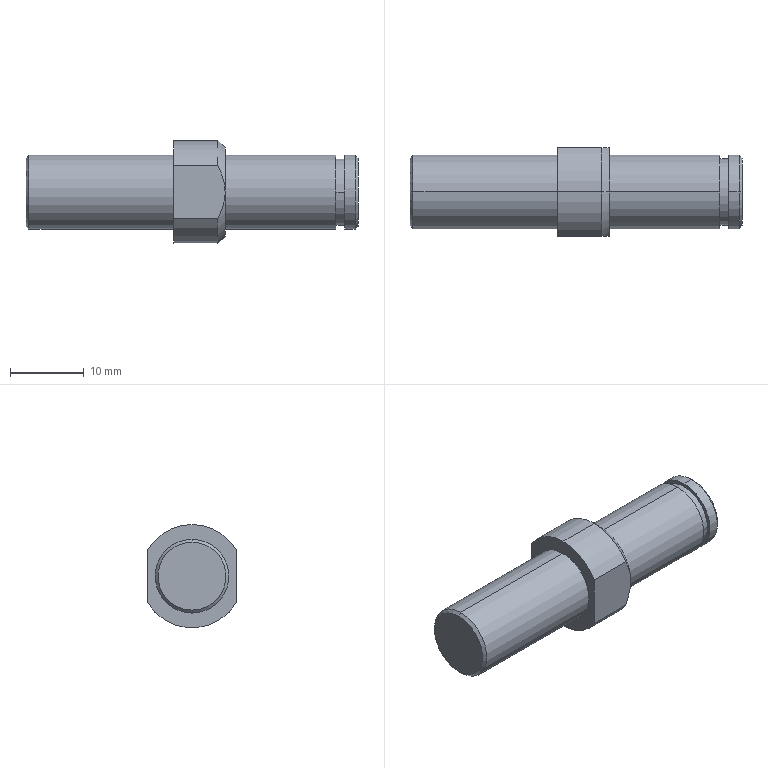Part | STEP file | 11-XSS11011 | 1 solid | 26 faces | box 45 x 12 x 14 mm | volume 3956 mm3 | cylinder 11 | plane 8 | cone 7 | commonest cylinder face diameters 10 x6 14 x3 9 x2
STEP:
#1=CARTESIAN_POINT('',(44.6,0.,5.));
#2=VERTEX_POINT('',#1);
#3=CARTESIAN_POINT('',(44.6,0.,-5.));
#4=VERTEX_POINT('',#3);
#5=CARTESIAN_POINT('',(44.6,0.,0.));
#6=DIRECTION('',(-1.,0.,0.));
#7=DIRECTION('',(0.,0.,-1.));
#8=AXIS2_PLACEMENT_3D('',#5,#6,#7);
#9=CIRCLE('',#8,5.);
#10=EDGE_CURVE('',#2,#4,#9,.T.);
#11=ORIENTED_EDGE('',*,*,#10,.T.);
#12=CARTESIAN_POINT('',(43.2,0.,-5.));
#13=VERTEX_POINT('',#12);
#14=CARTESIAN_POINT('',(0.,0.,-5.));
#15=DIRECTION('',(-1.,0.,0.));
#16=VECTOR('',#15,1000.);
#17=LINE('',#14,#16);
#18=EDGE_CURVE('',#4,#13,#17,.T.);
#19=ORIENTED_EDGE('',*,*,#18,.T.);
#20=CARTESIAN_POINT('',(43.2,0.,5.));
#21=VERTEX_POINT('',#20);
#22=CARTESIAN_POINT('',(43.2,0.,0.));
#23=DIRECTION('',(1.,0.,0.));
#24=DIRECTION('',(0.,1.,0.));
#25=AXIS2_PLACEMENT_3D('',#22,#23,#24);
#26=CIRCLE('',#25,5.);
#27=EDGE_CURVE('',#13,#21,#26,.T.);
#28=ORIENTED_EDGE('',*,*,#27,.T.);
#29=CARTESIAN_POINT('',(0.,0.,5.));
#30=DIRECTION('',(-1.,0.,0.));
#31=VECTOR('',#30,1000.);
#32=LINE('',#29,#31);
#33=EDGE_CURVE('',#2,#21,#32,.T.);
#34=ORIENTED_EDGE('',*,*,#33,.F.);
#35=EDGE_LOOP('',(#11,#19,#28,#34));
#36=FACE_OUTER_BOUND('',#35,.T.);
#37=CARTESIAN_POINT('',(0.,0.,0.));
#38=DIRECTION('',(-1.,0.,0.));
#39=DIRECTION('',(0.,0.,1.));
#40=AXIS2_PLACEMENT_3D('',#37,#38,#39);
#41=CYLINDRICAL_SURFACE('',#40,5.);
#42=ADVANCED_FACE('',(#36),#41,.T.);
#43=CARTESIAN_POINT('',(45.,0.,-4.6));
#44=VERTEX_POINT('',#43);
#45=CARTESIAN_POINT('',(45.,0.,4.6));
#46=VERTEX_POINT('',#45);
#47=CARTESIAN_POINT('',(45.,0.,0.));
#48=DIRECTION('',(1.,0.,0.));
#49=DIRECTION('',(0.,0.,-1.));
#50=AXIS2_PLACEMENT_3D('',#47,#48,#49);
#51=CIRCLE('',#50,4.6);
#52=EDGE_CURVE('',#44,#46,#51,.T.);
#53=ORIENTED_EDGE('',*,*,#52,.F.);
#54=CARTESIAN_POINT('',(44.6,0.,-5.));
#55=DIRECTION('',(-0.7071,0.,-0.7071));
#56=VECTOR('',#55,1000.);
#57=LINE('',#54,#56);
#58=EDGE_CURVE('',#44,#4,#57,.T.);
#59=ORIENTED_EDGE('',*,*,#58,.T.);
#60=ORIENTED_EDGE('',*,*,#10,.F.);
#61=CARTESIAN_POINT('',(44.6,0.,5.));
#62=DIRECTION('',(-0.7071,0.,0.7071));
#63=VECTOR('',#62,1000.);
#64=LINE('',#61,#63);
#65=EDGE_CURVE('',#46,#2,#64,.T.);
#66=ORIENTED_EDGE('',*,*,#65,.F.);
#67=EDGE_LOOP('',(#53,#59,#60,#66));
#68=FACE_OUTER_BOUND('',#67,.T.);
#69=CARTESIAN_POINT('',(44.6,0.,0.));
#70=DIRECTION('',(-1.,0.,0.));
#71=DIRECTION('',(0.,0.,1.));
#72=AXIS2_PLACEMENT_3D('',#69,#70,#71);
#73=CONICAL_SURFACE('',#72,5.,0.7854);
#74=ADVANCED_FACE('',(#68),#73,.T.);
#75=CARTESIAN_POINT('',(42.,4.5,0.));
#76=VERTEX_POINT('',#75);
#77=CARTESIAN_POINT('',(42.,-4.5,0.));
#78=VERTEX_POINT('',#77);
#79=CARTESIAN_POINT('',(42.,0.,0.));
#80=DIRECTION('',(1.,0.,0.));
#81=DIRECTION('',(0.,1.,0.));
#82=AXIS2_PLACEMENT_3D('',#79,#80,#81);
#83=CIRCLE('',#82,4.5);
#84=EDGE_CURVE('',#76,#78,#83,.T.);
#85=ORIENTED_EDGE('',*,*,#84,.T.);
#86=CARTESIAN_POINT('',(43.2,-4.5,0.));
#87=VERTEX_POINT('',#86);
#88=CARTESIAN_POINT('',(45.,-4.5,0.));
#89=DIRECTION('',(1.,0.,0.));
#90=VECTOR('',#89,1000.);
#91=LINE('',#88,#90);
#92=EDGE_CURVE('',#78,#87,#91,.T.);
#93=ORIENTED_EDGE('',*,*,#92,.T.);
#94=CARTESIAN_POINT('',(43.2,4.5,0.));
#95=VERTEX_POINT('',#94);
#96=CARTESIAN_POINT('',(43.2,0.,0.));
#97=DIRECTION('',(1.,0.,0.));
#98=DIRECTION('',(0.,1.,0.));
#99=AXIS2_PLACEMENT_3D('',#96,#97,#98);
#100=CIRCLE('',#99,4.5);
#101=EDGE_CURVE('',#95,#87,#100,.T.);
#102=ORIENTED_EDGE('',*,*,#101,.F.);
#103=CARTESIAN_POINT('',(45.,4.5,0.));
#104=DIRECTION('',(1.,0.,0.));
#105=VECTOR('',#104,1000.);
#106=LINE('',#103,#105);
#107=EDGE_CURVE('',#76,#95,#106,.T.);
#108=ORIENTED_EDGE('',*,*,#107,.F.);
#109=EDGE_LOOP('',(#85,#93,#102,#108));
#110=FACE_OUTER_BOUND('',#109,.T.);
#111=CARTESIAN_POINT('',(45.,0.,0.));
#112=DIRECTION('',(1.,0.,0.));
#113=DIRECTION('',(0.,1.,0.));
#114=AXIS2_PLACEMENT_3D('',#111,#112,#113);
#115=CYLINDRICAL_SURFACE('',#114,4.5);
#116=ADVANCED_FACE('',(#110),#115,.T.);
#117=CARTESIAN_POINT('',(27.,0.,6.));
#118=VERTEX_POINT('',#117);
#119=CARTESIAN_POINT('',(27.,-6.,0.));
#120=VERTEX_POINT('',#119);
#121=CARTESIAN_POINT('',(27.,0.,0.));
#122=DIRECTION('',(1.,0.,0.));
#123=DIRECTION('',(0.,0.,-1.));
#124=AXIS2_PLACEMENT_3D('',#121,#122,#123);
#125=CIRCLE('',#124,6.);
#126=EDGE_CURVE('',#118,#120,#125,.T.);
#127=ORIENTED_EDGE('',*,*,#126,.F.);
#128=CARTESIAN_POINT('',(26.,0.,7.));
#129=VERTEX_POINT('',#128);
#130=CARTESIAN_POINT('',(26.,0.,7.));
#131=DIRECTION('',(-0.7071,0.,0.7071));
#132=VECTOR('',#131,1000.);
#133=LINE('',#130,#132);
#134=EDGE_CURVE('',#118,#129,#133,.T.);
#135=ORIENTED_EDGE('',*,*,#134,.T.);
#136=CARTESIAN_POINT('',(26.,-6.,3.606));
#137=VERTEX_POINT('',#136);
#138=CARTESIAN_POINT('',(26.,0.,0.));
#139=DIRECTION('',(-1.,0.,0.));
#140=DIRECTION('',(0.,0.,-1.));
#141=AXIS2_PLACEMENT_3D('',#138,#139,#140);
#142=CIRCLE('',#141,7.);
#143=EDGE_CURVE('',#137,#129,#142,.T.);
#144=ORIENTED_EDGE('',*,*,#143,.F.);
#145=CARTESIAN_POINT('',(27.,-6.,0.));
#146=CARTESIAN_POINT('',(27.,-6.,0.6354));
#147=CARTESIAN_POINT('',(26.898,-6.,1.254));
#148=CARTESIAN_POINT('',(26.629,-6.,2.162));
#149=CARTESIAN_POINT('',(26.52,-6.,2.462));
#150=CARTESIAN_POINT('',(26.277,-6.,3.044));
#151=CARTESIAN_POINT('',(26.143,-6.,3.327));
#152=CARTESIAN_POINT('',(26.,-6.,3.606));
#153=B_SPLINE_CURVE_WITH_KNOTS('',3,(#145,#146,#147,#148,#149,#150,#151,#152),.UNSPECIFIED.,.F.,.F.,(4,2,2,4),(0.009642,0.01151,0.01245,0.01338),.UNSPECIFIED.);
#154=EDGE_CURVE('',#120,#137,#153,.T.);
#155=ORIENTED_EDGE('',*,*,#154,.F.);
#156=EDGE_LOOP('',(#127,#135,#144,#155));
#157=FACE_OUTER_BOUND('',#156,.T.);
#158=CARTESIAN_POINT('',(26.,0.,0.));
#159=DIRECTION('',(-1.,0.,0.));
#160=DIRECTION('',(0.,0.,1.));
#161=AXIS2_PLACEMENT_3D('',#158,#159,#160);
#162=CONICAL_SURFACE('',#161,7.,0.7854);
#163=ADVANCED_FACE('',(#157),#162,.T.);
#164=CARTESIAN_POINT('',(0.,0.,4.6));
#165=VERTEX_POINT('',#164);
#166=CARTESIAN_POINT('',(0.,0.,-4.6));
#167=VERTEX_POINT('',#166);
#168=CARTESIAN_POINT('',(0.,0.,0.));
#169=DIRECTION('',(-1.,0.,0.));
#170=DIRECTION('',(0.,0.,1.));
#171=AXIS2_PLACEMENT_3D('',#168,#169,#170);
#172=CIRCLE('',#171,4.6);
#173=EDGE_CURVE('',#165,#167,#172,.T.);
#174=ORIENTED_EDGE('',*,*,#173,.F.);
#175=CARTESIAN_POINT('',(0.4,0.,5.));
#176=VERTEX_POINT('',#175);
#177=CARTESIAN_POINT('',(0.,0.,4.6));
#178=DIRECTION('',(0.7071,0.,0.7071));
#179=VECTOR('',#178,1000.);
#180=LINE('',#177,#179);
#181=EDGE_CURVE('',#165,#176,#180,.T.);
#182=ORIENTED_EDGE('',*,*,#181,.T.);
#183=CARTESIAN_POINT('',(0.4,0.,-5.));
#184=VERTEX_POINT('',#183);
#185=CARTESIAN_POINT('',(0.4,0.,0.));
#186=DIRECTION('',(1.,0.,0.));
#187=DIRECTION('',(0.,0.,1.));
#188=AXIS2_PLACEMENT_3D('',#185,#186,#187);
#189=CIRCLE('',#188,5.);
#190=EDGE_CURVE('',#184,#176,#189,.T.);
#191=ORIENTED_EDGE('',*,*,#190,.F.);
#192=CARTESIAN_POINT('',(0.,0.,-4.6));
#193=DIRECTION('',(0.7071,0.,-0.7071));
#194=VECTOR('',#193,1000.);
#195=LINE('',#192,#194);
#196=EDGE_CURVE('',#167,#184,#195,.T.);
#197=ORIENTED_EDGE('',*,*,#196,.F.);
#198=EDGE_LOOP('',(#174,#182,#191,#197));
#199=FACE_OUTER_BOUND('',#198,.T.);
#200=CARTESIAN_POINT('',(0.,0.,0.));
#201=DIRECTION('',(1.,0.,0.));
#202=DIRECTION('',(0.,0.,-1.));
#203=AXIS2_PLACEMENT_3D('',#200,#201,#202);
#204=CONICAL_SURFACE('',#203,4.6,0.7854);
#205=ADVANCED_FACE('',(#199),#204,.T.);
#206=CARTESIAN_POINT('',(42.,0.,-5.));
#207=VERTEX_POINT('',#206);
#208=CARTESIAN_POINT('',(42.,0.,5.));
#209=VERTEX_POINT('',#208);
#210=CARTESIAN_POINT('',(42.,0.,0.));
#211=DIRECTION('',(1.,0.,0.));
#212=DIRECTION('',(0.,1.,0.));
#213=AXIS2_PLACEMENT_3D('',#210,#211,#212);
#214=CIRCLE('',#213,5.);
#215=EDGE_CURVE('',#207,#209,#214,.T.);
#216=ORIENTED_EDGE('',*,*,#215,.F.);
#217=CARTESIAN_POINT('',(27.,0.,-5.));
#218=VERTEX_POINT('',#217);
#219=CARTESIAN_POINT('',(0.,0.,-5.));
#220=DIRECTION('',(-1.,0.,0.));
#221=VECTOR('',#220,1000.);
#222=LINE('',#219,#221);
#223=EDGE_CURVE('',#207,#218,#222,.T.);
#224=ORIENTED_EDGE('',*,*,#223,.T.);
#225=CARTESIAN_POINT('',(27.,0.,5.));
#226=VERTEX_POINT('',#225);
#227=CARTESIAN_POINT('',(27.,0.,0.));
#228=DIRECTION('',(-1.,0.,0.));
#229=DIRECTION('',(0.,0.,1.));
#230=AXIS2_PLACEMENT_3D('',#227,#228,#229);
#231=CIRCLE('',#230,5.);
#232=EDGE_CURVE('',#226,#218,#231,.T.);
#233=ORIENTED_EDGE('',*,*,#232,.F.);
#234=CARTESIAN_POINT('',(0.,0.,5.));
#235=DIRECTION('',(-1.,0.,0.));
#236=VECTOR('',#235,1000.);
#237=LINE('',#234,#236);
#238=EDGE_CURVE('',#209,#226,#237,.T.);
#239=ORIENTED_EDGE('',*,*,#238,.F.);
#240=EDGE_LOOP('',(#216,#224,#233,#239));
#241=FACE_OUTER_BOUND('',#240,.T.);
#242=CARTESIAN_POINT('',(0.,0.,0.));
#243=DIRECTION('',(-1.,0.,0.));
#244=DIRECTION('',(0.,0.,1.));
#245=AXIS2_PLACEMENT_3D('',#242,#243,#244);
#246=CYLINDRICAL_SURFACE('',#245,5.);
#247=ADVANCED_FACE('',(#241),#246,.T.);
#248=CARTESIAN_POINT('',(20.,0.,5.));
#249=VERTEX_POINT('',#248);
#250=CARTESIAN_POINT('',(20.,0.,-5.));
#251=VERTEX_POINT('',#250);
#252=CARTESIAN_POINT('',(20.,0.,0.));
#253=DIRECTION('',(-1.,0.,0.));
#254=DIRECTION('',(0.,0.,1.));
#255=AXIS2_PLACEMENT_3D('',#252,#253,#254);
#256=CIRCLE('',#255,5.);
#257=EDGE_CURVE('',#249,#251,#256,.T.);
#258=ORIENTED_EDGE('',*,*,#257,.T.);
#259=CARTESIAN_POINT('',(0.,0.,-5.));
#260=DIRECTION('',(-1.,0.,0.));
#261=VECTOR('',#260,1000.);
#262=LINE('',#259,#261);
#263=EDGE_CURVE('',#251,#184,#262,.T.);
#264=ORIENTED_EDGE('',*,*,#263,.T.);
#265=ORIENTED_EDGE('',*,*,#190,.T.);
#266=CARTESIAN_POINT('',(0.,0.,5.));
#267=DIRECTION('',(-1.,0.,0.));
#268=VECTOR('',#267,1000.);
#269=LINE('',#266,#268);
#270=EDGE_CURVE('',#249,#176,#269,.T.);
#271=ORIENTED_EDGE('',*,*,#270,.F.);
#272=EDGE_LOOP('',(#258,#264,#265,#271));
#273=FACE_OUTER_BOUND('',#272,.T.);
#274=CARTESIAN_POINT('',(0.,0.,0.));
#275=DIRECTION('',(-1.,0.,0.));
#276=DIRECTION('',(0.,0.,1.));
#277=AXIS2_PLACEMENT_3D('',#274,#275,#276);
#278=CYLINDRICAL_SURFACE('',#277,5.);
#279=ADVANCED_FACE('',(#273),#278,.T.);
#280=ORIENTED_EDGE('',*,*,#143,.T.);
#281=CARTESIAN_POINT('',(20.,0.,7.));
#282=VERTEX_POINT('',#281);
#283=CARTESIAN_POINT('',(0.,0.,7.));
#284=DIRECTION('',(-1.,0.,0.));
#285=VECTOR('',#284,1000.);
#286=LINE('',#283,#285);
#287=EDGE_CURVE('',#129,#282,#286,.T.);
#288=ORIENTED_EDGE('',*,*,#287,.T.);
#289=CARTESIAN_POINT('',(20.,-6.,3.606));
#290=VERTEX_POINT('',#289);
#291=CARTESIAN_POINT('',(20.,0.,0.));
#292=DIRECTION('',(-1.,0.,0.));
#293=DIRECTION('',(0.,0.,1.));
#294=AXIS2_PLACEMENT_3D('',#291,#292,#293);
#295=CIRCLE('',#294,7.);
#296=EDGE_CURVE('',#290,#282,#295,.T.);
#297=ORIENTED_EDGE('',*,*,#296,.F.);
#298=CARTESIAN_POINT('',(45.,-6.,3.606));
#299=DIRECTION('',(-1.,0.,0.));
#300=VECTOR('',#299,1000.);
#301=LINE('',#298,#300);
#302=EDGE_CURVE('',#137,#290,#301,.T.);
#303=ORIENTED_EDGE('',*,*,#302,.F.);
#304=EDGE_LOOP('',(#280,#288,#297,#303));
#305=FACE_OUTER_BOUND('',#304,.T.);
#306=CARTESIAN_POINT('',(0.,0.,0.));
#307=DIRECTION('',(-1.,0.,0.));
#308=DIRECTION('',(0.,0.,1.));
#309=AXIS2_PLACEMENT_3D('',#306,#307,#308);
#310=CYLINDRICAL_SURFACE('',#309,7.);
#311=ADVANCED_FACE('',(#305),#310,.T.);
#312=ORIENTED_EDGE('',*,*,#287,.F.);
#313=CARTESIAN_POINT('',(26.,6.,3.606));
#314=VERTEX_POINT('',#313);
#315=CARTESIAN_POINT('',(26.,0.,0.));
#316=DIRECTION('',(-1.,0.,0.));
#317=DIRECTION('',(0.,0.,-1.));
#318=AXIS2_PLACEMENT_3D('',#315,#316,#317);
#319=CIRCLE('',#318,7.);
#320=EDGE_CURVE('',#129,#314,#319,.T.);
#321=ORIENTED_EDGE('',*,*,#320,.T.);
#322=CARTESIAN_POINT('',(20.,6.,3.606));
#323=VERTEX_POINT('',#322);
#324=CARTESIAN_POINT('',(45.,6.,3.606));
#325=DIRECTION('',(-1.,0.,0.));
#326=VECTOR('',#325,1000.);
#327=LINE('',#324,#326);
#328=EDGE_CURVE('',#314,#323,#327,.T.);
#329=ORIENTED_EDGE('',*,*,#328,.T.);
#330=CARTESIAN_POINT('',(20.,0.,0.));
#331=DIRECTION('',(-1.,0.,0.));
#332=DIRECTION('',(0.,0.,1.));
#333=AXIS2_PLACEMENT_3D('',#330,#331,#332);
#334=CIRCLE('',#333,7.);
#335=EDGE_CURVE('',#282,#323,#334,.T.);
#336=ORIENTED_EDGE('',*,*,#335,.F.);
#337=EDGE_LOOP('',(#312,#321,#329,#336));
#338=FACE_OUTER_BOUND('',#337,.T.);
#339=CARTESIAN_POINT('',(0.,0.,0.));
#340=DIRECTION('',(-1.,0.,0.));
#341=DIRECTION('',(0.,0.,1.));
#342=AXIS2_PLACEMENT_3D('',#339,#340,#341);
#343=CYLINDRICAL_SURFACE('',#342,7.);
#344=ADVANCED_FACE('',(#338),#343,.T.);
#345=CARTESIAN_POINT('',(26.,-6.,-3.606));
#346=VERTEX_POINT('',#345);
#347=CARTESIAN_POINT('',(26.,-6.,-3.606));
#348=CARTESIAN_POINT('',(26.143,-6.,-3.327));
#349=CARTESIAN_POINT('',(26.278,-6.,-3.043));
#350=CARTESIAN_POINT('',(26.521,-6.,-2.458));
#351=CARTESIAN_POINT('',(26.629,-6.,-2.161));
#352=CARTESIAN_POINT('',(26.807,-6.,-1.56));
#353=CARTESIAN_POINT('',(26.878,-6.,-1.255));
#354=CARTESIAN_POINT('',(26.974,-6.,-0.635));
#355=CARTESIAN_POINT('',(27.,-6.,-0.3173));
#356=CARTESIAN_POINT('',(27.,-6.,0.));
#357=B_SPLINE_CURVE_WITH_KNOTS('',3,(#347,#348,#349,#350,#351,#352,#353,#354,#355,#356),.UNSPECIFIED.,.F.,.F.,(4,2,2,2,4),(0.005907,0.006841,0.007775,0.008708,0.009642),.UNSPECIFIED.);
#358=EDGE_CURVE('',#346,#120,#357,.T.);
#359=ORIENTED_EDGE('',*,*,#358,.F.);
#360=CARTESIAN_POINT('',(26.,6.,-3.606));
#361=VERTEX_POINT('',#360);
#362=CARTESIAN_POINT('',(26.,0.,0.));
#363=DIRECTION('',(-1.,0.,0.));
#364=DIRECTION('',(0.,0.,-1.));
#365=AXIS2_PLACEMENT_3D('',#362,#363,#364);
#366=CIRCLE('',#365,7.);
#367=EDGE_CURVE('',#361,#346,#366,.T.);
#368=ORIENTED_EDGE('',*,*,#367,.F.);
#369=CARTESIAN_POINT('',(27.,6.,0.));
#370=VERTEX_POINT('',#369);
#371=CARTESIAN_POINT('',(27.,6.,0.));
#372=CARTESIAN_POINT('',(27.,6.,-0.3173));
#373=CARTESIAN_POINT('',(26.974,6.,-0.635));
#374=CARTESIAN_POINT('',(26.878,6.,-1.255));
#375=CARTESIAN_POINT('',(26.807,6.,-1.56));
#376=CARTESIAN_POINT('',(26.629,6.,-2.161));
#377=CARTESIAN_POINT('',(26.521,6.,-2.458));
#378=CARTESIAN_POINT('',(26.278,6.,-3.043));
#379=CARTESIAN_POINT('',(26.143,6.,-3.327));
#380=CARTESIAN_POINT('',(26.,6.,-3.606));
#381=B_SPLINE_CURVE_WITH_KNOTS('',3,(#371,#372,#373,#374,#375,#376,#377,#378,#379,#380),.UNSPECIFIED.,.F.,.F.,(4,2,2,2,4),(0.007237,0.008174,0.009111,0.01005,0.01098),.UNSPECIFIED.);
#382=EDGE_CURVE('',#370,#361,#381,.T.);
#383=ORIENTED_EDGE('',*,*,#382,.F.);
#384=CARTESIAN_POINT('',(27.,0.,0.));
#385=DIRECTION('',(1.,0.,0.));
#386=DIRECTION('',(0.,0.,-1.));
#387=AXIS2_PLACEMENT_3D('',#384,#385,#386);
#388=CIRCLE('',#387,6.);
#389=EDGE_CURVE('',#120,#370,#388,.T.);
#390=ORIENTED_EDGE('',*,*,#389,.F.);
#391=EDGE_LOOP('',(#359,#368,#383,#390));
#392=FACE_OUTER_BOUND('',#391,.T.);
#393=CARTESIAN_POINT('',(26.,0.,0.));
#394=DIRECTION('',(-1.,0.,0.));
#395=DIRECTION('',(0.,0.,1.));
#396=AXIS2_PLACEMENT_3D('',#393,#394,#395);
#397=CONICAL_SURFACE('',#396,7.,0.7854);
#398=ADVANCED_FACE('',(#392),#397,.T.);
#399=CARTESIAN_POINT('',(0.,0.,0.));
#400=DIRECTION('',(-1.,0.,0.));
#401=DIRECTION('',(0.,0.,1.));
#402=AXIS2_PLACEMENT_3D('',#399,#400,#401);
#403=CIRCLE('',#402,4.6);
#404=EDGE_CURVE('',#167,#165,#403,.T.);
#405=ORIENTED_EDGE('',*,*,#404,.T.);
#406=ORIENTED_EDGE('',*,*,#173,.T.);
#407=EDGE_LOOP('',(#405,#406));
#408=FACE_OUTER_BOUND('',#407,.T.);
#409=CARTESIAN_POINT('',(0.,0.,0.));
#410=DIRECTION('',(-1.,0.,0.));
#411=DIRECTION('',(0.,0.,1.));
#412=AXIS2_PLACEMENT_3D('',#409,#410,#411);
#413=PLANE('',#412);
#414=ADVANCED_FACE('',(#408),#413,.T.);
#415=ORIENTED_EDGE('',*,*,#263,.F.);
#416=CARTESIAN_POINT('',(20.,0.,0.));
#417=DIRECTION('',(-1.,0.,0.));
#418=DIRECTION('',(0.,0.,1.));
#419=AXIS2_PLACEMENT_3D('',#416,#417,#418);
#420=CIRCLE('',#419,5.);
#421=EDGE_CURVE('',#251,#249,#420,.T.);
#422=ORIENTED_EDGE('',*,*,#421,.T.);
#423=ORIENTED_EDGE('',*,*,#270,.T.);
#424=CARTESIAN_POINT('',(0.4,0.,0.));
#425=DIRECTION('',(1.,0.,0.));
#426=DIRECTION('',(0.,0.,1.));
#427=AXIS2_PLACEMENT_3D('',#424,#425,#426);
#428=CIRCLE('',#427,5.);
#429=EDGE_CURVE('',#176,#184,#428,.T.);
#430=ORIENTED_EDGE('',*,*,#429,.T.);
#431=EDGE_LOOP('',(#415,#422,#423,#430));
#432=FACE_OUTER_BOUND('',#431,.T.);
#433=CARTESIAN_POINT('',(0.,0.,0.));
#434=DIRECTION('',(-1.,0.,0.));
#435=DIRECTION('',(0.,0.,1.));
#436=AXIS2_PLACEMENT_3D('',#433,#434,#435);
#437=CYLINDRICAL_SURFACE('',#436,5.);
#438=ADVANCED_FACE('',(#432),#437,.T.);
#439=CARTESIAN_POINT('',(20.,-6.,-3.606));
#440=VERTEX_POINT('',#439);
#441=CARTESIAN_POINT('',(20.,-6.,-3.606));
#442=DIRECTION('',(0.,0.,-1.));
#443=VECTOR('',#442,1000.);
#444=LINE('',#441,#443);
#445=EDGE_CURVE('',#290,#440,#444,.T.);
#446=ORIENTED_EDGE('',*,*,#445,.F.);
#447=ORIENTED_EDGE('',*,*,#296,.T.);
#448=ORIENTED_EDGE('',*,*,#335,.T.);
#449=CARTESIAN_POINT('',(20.,6.,-3.606));
#450=VERTEX_POINT('',#449);
#451=CARTESIAN_POINT('',(20.,6.,-3.606));
#452=DIRECTION('',(0.,0.,1.));
#453=VECTOR('',#452,1000.);
#454=LINE('',#451,#453);
#455=EDGE_CURVE('',#450,#323,#454,.T.);
#456=ORIENTED_EDGE('',*,*,#455,.F.);
#457=CARTESIAN_POINT('',(20.,0.,0.));
#458=DIRECTION('',(-1.,0.,0.));
#459=DIRECTION('',(0.,0.,1.));
#460=AXIS2_PLACEMENT_3D('',#457,#458,#459);
#461=CIRCLE('',#460,7.);
#462=EDGE_CURVE('',#450,#440,#461,.T.);
#463=ORIENTED_EDGE('',*,*,#462,.T.);
#464=EDGE_LOOP('',(#446,#447,#448,#456,#463));
#465=FACE_OUTER_BOUND('',#464,.T.);
#466=ORIENTED_EDGE('',*,*,#257,.F.);
#467=ORIENTED_EDGE('',*,*,#421,.F.);
#468=EDGE_LOOP('',(#466,#467));
#469=FACE_BOUND('',#468,.T.);
#470=CARTESIAN_POINT('',(20.,0.,5.));
#471=DIRECTION('',(-1.,0.,0.));
#472=DIRECTION('',(0.,0.,1.));
#473=AXIS2_PLACEMENT_3D('',#470,#471,#472);
#474=PLANE('',#473);
#475=ADVANCED_FACE('',(#465,#469),#474,.T.);
#476=CARTESIAN_POINT('',(45.,-6.,-3.606));
#477=DIRECTION('',(-1.,0.,0.));
#478=VECTOR('',#477,1000.);
#479=LINE('',#476,#478);
#480=EDGE_CURVE('',#346,#440,#479,.T.);
#481=ORIENTED_EDGE('',*,*,#480,.T.);
#482=ORIENTED_EDGE('',*,*,#462,.F.);
#483=CARTESIAN_POINT('',(45.,6.,-3.606));
#484=DIRECTION('',(-1.,0.,0.));
#485=VECTOR('',#484,1000.);
#486=LINE('',#483,#485);
#487=EDGE_CURVE('',#361,#450,#486,.T.);
#488=ORIENTED_EDGE('',*,*,#487,.F.);
#489=ORIENTED_EDGE('',*,*,#367,.T.);
#490=EDGE_LOOP('',(#481,#482,#488,#489));
#491=FACE_OUTER_BOUND('',#490,.T.);
#492=CARTESIAN_POINT('',(0.,0.,0.));
#493=DIRECTION('',(-1.,0.,0.));
#494=DIRECTION('',(0.,0.,1.));
#495=AXIS2_PLACEMENT_3D('',#492,#493,#494);
#496=CYLINDRICAL_SURFACE('',#495,7.);
#497=ADVANCED_FACE('',(#491),#496,.T.);
#498=CARTESIAN_POINT('',(27.,0.,0.));
#499=DIRECTION('',(1.,0.,0.));
#500=DIRECTION('',(0.,0.,-1.));
#501=AXIS2_PLACEMENT_3D('',#498,#499,#500);
#502=CIRCLE('',#501,6.);
#503=EDGE_CURVE('',#370,#118,#502,.T.);
#504=ORIENTED_EDGE('',*,*,#503,.T.);
#505=ORIENTED_EDGE('',*,*,#126,.T.);
#506=ORIENTED_EDGE('',*,*,#389,.T.);
#507=EDGE_LOOP('',(#504,#505,#506));
#508=FACE_OUTER_BOUND('',#507,.T.);
#509=ORIENTED_EDGE('',*,*,#232,.T.);
#510=CARTESIAN_POINT('',(27.,0.,0.));
#511=DIRECTION('',(-1.,0.,0.));
#512=DIRECTION('',(0.,0.,1.));
#513=AXIS2_PLACEMENT_3D('',#510,#511,#512);
#514=CIRCLE('',#513,5.);
#515=EDGE_CURVE('',#218,#226,#514,.T.);
#516=ORIENTED_EDGE('',*,*,#515,.T.);
#517=EDGE_LOOP('',(#509,#516));
#518=FACE_BOUND('',#517,.T.);
#519=CARTESIAN_POINT('',(27.,0.,7.));
#520=DIRECTION('',(1.,0.,0.));
#521=DIRECTION('',(0.,0.,-1.));
#522=AXIS2_PLACEMENT_3D('',#519,#520,#521);
#523=PLANE('',#522);
#524=ADVANCED_FACE('',(#508,#518),#523,.T.);
#525=ORIENTED_EDGE('',*,*,#223,.F.);
#526=CARTESIAN_POINT('',(42.,0.,0.));
#527=DIRECTION('',(1.,0.,0.));
#528=DIRECTION('',(0.,1.,0.));
#529=AXIS2_PLACEMENT_3D('',#526,#527,#528);
#530=CIRCLE('',#529,5.);
#531=EDGE_CURVE('',#209,#207,#530,.T.);
#532=ORIENTED_EDGE('',*,*,#531,.F.);
#533=ORIENTED_EDGE('',*,*,#238,.T.);
#534=ORIENTED_EDGE('',*,*,#515,.F.);
#535=EDGE_LOOP('',(#525,#532,#533,#534));
#536=FACE_OUTER_BOUND('',#535,.T.);
#537=CARTESIAN_POINT('',(0.,0.,0.));
#538=DIRECTION('',(-1.,0.,0.));
#539=DIRECTION('',(0.,0.,1.));
#540=AXIS2_PLACEMENT_3D('',#537,#538,#539);
#541=CYLINDRICAL_SURFACE('',#540,5.);
#542=ADVANCED_FACE('',(#536),#541,.T.);
#543=ORIENTED_EDGE('',*,*,#181,.F.);
#544=ORIENTED_EDGE('',*,*,#404,.F.);
#545=ORIENTED_EDGE('',*,*,#196,.T.);
#546=ORIENTED_EDGE('',*,*,#429,.F.);
#547=EDGE_LOOP('',(#543,#544,#545,#546));
#548=FACE_OUTER_BOUND('',#547,.T.);
#549=CARTESIAN_POINT('',(0.,0.,0.));
#550=DIRECTION('',(1.,0.,0.));
#551=DIRECTION('',(0.,0.,-1.));
#552=AXIS2_PLACEMENT_3D('',#549,#550,#551);
#553=CONICAL_SURFACE('',#552,4.6,0.7854);
#554=ADVANCED_FACE('',(#548),#553,.T.);
#555=ORIENTED_EDGE('',*,*,#134,.F.);
#556=ORIENTED_EDGE('',*,*,#503,.F.);
#557=CARTESIAN_POINT('',(26.,6.,3.606));
#558=CARTESIAN_POINT('',(26.143,6.,3.327));
#559=CARTESIAN_POINT('',(26.277,6.,3.044));
#560=CARTESIAN_POINT('',(26.52,6.,2.462));
#561=CARTESIAN_POINT('',(26.629,6.,2.162));
#562=CARTESIAN_POINT('',(26.898,6.,1.254));
#563=CARTESIAN_POINT('',(27.,6.,0.6354));
#564=CARTESIAN_POINT('',(27.,6.,0.));
#565=B_SPLINE_CURVE_WITH_KNOTS('',3,(#557,#558,#559,#560,#561,#562,#563,#564),.UNSPECIFIED.,.F.,.F.,(4,2,2,4),(0.003487,0.004425,0.005362,0.007237),.UNSPECIFIED.);
#566=EDGE_CURVE('',#314,#370,#565,.T.);
#567=ORIENTED_EDGE('',*,*,#566,.F.);
#568=ORIENTED_EDGE('',*,*,#320,.F.);
#569=EDGE_LOOP('',(#555,#556,#567,#568));
#570=FACE_OUTER_BOUND('',#569,.T.);
#571=CARTESIAN_POINT('',(26.,0.,0.));
#572=DIRECTION('',(-1.,0.,0.));
#573=DIRECTION('',(0.,0.,1.));
#574=AXIS2_PLACEMENT_3D('',#571,#572,#573);
#575=CONICAL_SURFACE('',#574,7.,0.7854);
#576=ADVANCED_FACE('',(#570),#575,.T.);
#577=ORIENTED_EDGE('',*,*,#566,.T.);
#578=ORIENTED_EDGE('',*,*,#382,.T.);
#579=ORIENTED_EDGE('',*,*,#487,.T.);
#580=ORIENTED_EDGE('',*,*,#455,.T.);
#581=ORIENTED_EDGE('',*,*,#328,.F.);
#582=EDGE_LOOP('',(#577,#578,#579,#580,#581));
#583=FACE_OUTER_BOUND('',#582,.T.);
#584=CARTESIAN_POINT('',(45.,6.,-3.606));
#585=DIRECTION('',(0.,-1.,0.));
#586=DIRECTION('',(0.,0.,-1.));
#587=AXIS2_PLACEMENT_3D('',#584,#585,#586);
#588=PLANE('',#587);
#589=ADVANCED_FACE('',(#583),#588,.F.);
#590=ORIENTED_EDGE('',*,*,#358,.T.);
#591=ORIENTED_EDGE('',*,*,#154,.T.);
#592=ORIENTED_EDGE('',*,*,#302,.T.);
#593=ORIENTED_EDGE('',*,*,#445,.T.);
#594=ORIENTED_EDGE('',*,*,#480,.F.);
#595=EDGE_LOOP('',(#590,#591,#592,#593,#594));
#596=FACE_OUTER_BOUND('',#595,.T.);
#597=CARTESIAN_POINT('',(45.,-6.,-3.606));
#598=DIRECTION('',(0.,1.,0.));
#599=DIRECTION('',(0.,0.,1.));
#600=AXIS2_PLACEMENT_3D('',#597,#598,#599);
#601=PLANE('',#600);
#602=ADVANCED_FACE('',(#596),#601,.F.);
#603=CARTESIAN_POINT('',(43.2,0.,0.));
#604=DIRECTION('',(1.,0.,0.));
#605=DIRECTION('',(0.,1.,0.));
#606=AXIS2_PLACEMENT_3D('',#603,#604,#605);
#607=CIRCLE('',#606,5.);
#608=EDGE_CURVE('',#21,#13,#607,.T.);
#609=ORIENTED_EDGE('',*,*,#608,.F.);
#610=ORIENTED_EDGE('',*,*,#27,.F.);
#611=EDGE_LOOP('',(#609,#610));
#612=FACE_OUTER_BOUND('',#611,.T.);
#613=ORIENTED_EDGE('',*,*,#101,.T.);
#614=CARTESIAN_POINT('',(43.2,0.,0.));
#615=DIRECTION('',(1.,0.,0.));
#616=DIRECTION('',(0.,1.,0.));
#617=AXIS2_PLACEMENT_3D('',#614,#615,#616);
#618=CIRCLE('',#617,4.5);
#619=EDGE_CURVE('',#87,#95,#618,.T.);
#620=ORIENTED_EDGE('',*,*,#619,.T.);
#621=EDGE_LOOP('',(#613,#620));
#622=FACE_BOUND('',#621,.T.);
#623=CARTESIAN_POINT('',(43.2,5.,0.));
#624=DIRECTION('',(1.,0.,0.));
#625=DIRECTION('',(0.,1.,0.));
#626=AXIS2_PLACEMENT_3D('',#623,#624,#625);
#627=PLANE('',#626);
#628=ADVANCED_FACE('',(#612,#622),#627,.F.);
#629=ORIENTED_EDGE('',*,*,#92,.F.);
#630=CARTESIAN_POINT('',(42.,0.,0.));
#631=DIRECTION('',(1.,0.,0.));
#632=DIRECTION('',(0.,1.,0.));
#633=AXIS2_PLACEMENT_3D('',#630,#631,#632);
#634=CIRCLE('',#633,4.5);
#635=EDGE_CURVE('',#78,#76,#634,.T.);
#636=ORIENTED_EDGE('',*,*,#635,.T.);
#637=ORIENTED_EDGE('',*,*,#107,.T.);
#638=ORIENTED_EDGE('',*,*,#619,.F.);
#639=EDGE_LOOP('',(#629,#636,#637,#638));
#640=FACE_OUTER_BOUND('',#639,.T.);
#641=CARTESIAN_POINT('',(45.,0.,0.));
#642=DIRECTION('',(1.,0.,0.));
#643=DIRECTION('',(0.,1.,0.));
#644=AXIS2_PLACEMENT_3D('',#641,#642,#643);
#645=CYLINDRICAL_SURFACE('',#644,4.5);
#646=ADVANCED_FACE('',(#640),#645,.T.);
#647=ORIENTED_EDGE('',*,*,#84,.F.);
#648=ORIENTED_EDGE('',*,*,#635,.F.);
#649=EDGE_LOOP('',(#647,#648));
#650=FACE_BOUND('',#649,.T.);
#651=ORIENTED_EDGE('',*,*,#531,.T.);
#652=ORIENTED_EDGE('',*,*,#215,.T.);
#653=EDGE_LOOP('',(#651,#652));
#654=FACE_OUTER_BOUND('',#653,.T.);
#655=CARTESIAN_POINT('',(42.,5.,0.));
#656=DIRECTION('',(-1.,0.,0.));
#657=DIRECTION('',(0.,-1.,0.));
#658=AXIS2_PLACEMENT_3D('',#655,#656,#657);
#659=PLANE('',#658);
#660=ADVANCED_FACE('',(#650,#654),#659,.F.);
#661=CARTESIAN_POINT('',(45.,0.,0.));
#662=DIRECTION('',(1.,0.,0.));
#663=DIRECTION('',(0.,0.,-1.));
#664=AXIS2_PLACEMENT_3D('',#661,#662,#663);
#665=CIRCLE('',#664,4.6);
#666=EDGE_CURVE('',#46,#44,#665,.T.);
#667=ORIENTED_EDGE('',*,*,#666,.T.);
#668=ORIENTED_EDGE('',*,*,#52,.T.);
#669=EDGE_LOOP('',(#667,#668));
#670=FACE_OUTER_BOUND('',#669,.T.);
#671=CARTESIAN_POINT('',(45.,0.,5.));
#672=DIRECTION('',(1.,0.,0.));
#673=DIRECTION('',(0.,0.,-1.));
#674=AXIS2_PLACEMENT_3D('',#671,#672,#673);
#675=PLANE('',#674);
#676=ADVANCED_FACE('',(#670),#675,.T.);
#677=ORIENTED_EDGE('',*,*,#58,.F.);
#678=ORIENTED_EDGE('',*,*,#666,.F.);
#679=ORIENTED_EDGE('',*,*,#65,.T.);
#680=CARTESIAN_POINT('',(44.6,0.,0.));
#681=DIRECTION('',(-1.,0.,0.));
#682=DIRECTION('',(0.,0.,-1.));
#683=AXIS2_PLACEMENT_3D('',#680,#681,#682);
#684=CIRCLE('',#683,5.);
#685=EDGE_CURVE('',#4,#2,#684,.T.);
#686=ORIENTED_EDGE('',*,*,#685,.F.);
#687=EDGE_LOOP('',(#677,#678,#679,#686));
#688=FACE_OUTER_BOUND('',#687,.T.);
#689=CARTESIAN_POINT('',(44.6,0.,0.));
#690=DIRECTION('',(-1.,0.,0.));
#691=DIRECTION('',(0.,0.,1.));
#692=AXIS2_PLACEMENT_3D('',#689,#690,#691);
#693=CONICAL_SURFACE('',#692,5.,0.7854);
#694=ADVANCED_FACE('',(#688),#693,.T.);
#695=ORIENTED_EDGE('',*,*,#18,.F.);
#696=ORIENTED_EDGE('',*,*,#685,.T.);
#697=ORIENTED_EDGE('',*,*,#33,.T.);
#698=ORIENTED_EDGE('',*,*,#608,.T.);
#699=EDGE_LOOP('',(#695,#696,#697,#698));
#700=FACE_OUTER_BOUND('',#699,.T.);
#701=CARTESIAN_POINT('',(0.,0.,0.));
#702=DIRECTION('',(-1.,0.,0.));
#703=DIRECTION('',(0.,0.,1.));
#704=AXIS2_PLACEMENT_3D('',#701,#702,#703);
#705=CYLINDRICAL_SURFACE('',#704,5.);
#706=ADVANCED_FACE('',(#700),#705,.T.);
#707=CLOSED_SHELL('',(#42,#74,#116,#163,#205,#247,#279,#311,#344,#398,#414,#438,#475,#497,#524,#542,#554,#576,#589,#602,#628,#646,#660,#676,#694,#706));
#708=MANIFOLD_SOLID_BREP('',#707);
#709=CARTESIAN_POINT('',(0.,0.,0.));
#710=DIRECTION('',(0.,0.,1.));
#711=DIRECTION('',(1.,0.,0.));
#712=AXIS2_PLACEMENT_3D('',#709,#710,#711);
#713=(LENGTH_UNIT()NAMED_UNIT(*)SI_UNIT(.MILLI.,.METRE.));
#714=UNCERTAINTY_MEASURE_WITH_UNIT(LENGTH_MEASURE(0.00001),#713,'','');
#715=(NAMED_UNIT(*)PLANE_ANGLE_UNIT()SI_UNIT($,.RADIAN.));
#716=(NAMED_UNIT(*)SI_UNIT($,.STERADIAN.)SOLID_ANGLE_UNIT());
#717=(GEOMETRIC_REPRESENTATION_CONTEXT(3)GLOBAL_UNCERTAINTY_ASSIGNED_CONTEXT((#714))GLOBAL_UNIT_ASSIGNED_CONTEXT((#713,#715,#716))REPRESENTATION_CONTEXT('',''));
#718=ADVANCED_BREP_SHAPE_REPRESENTATION('',(#708,#712),#717);